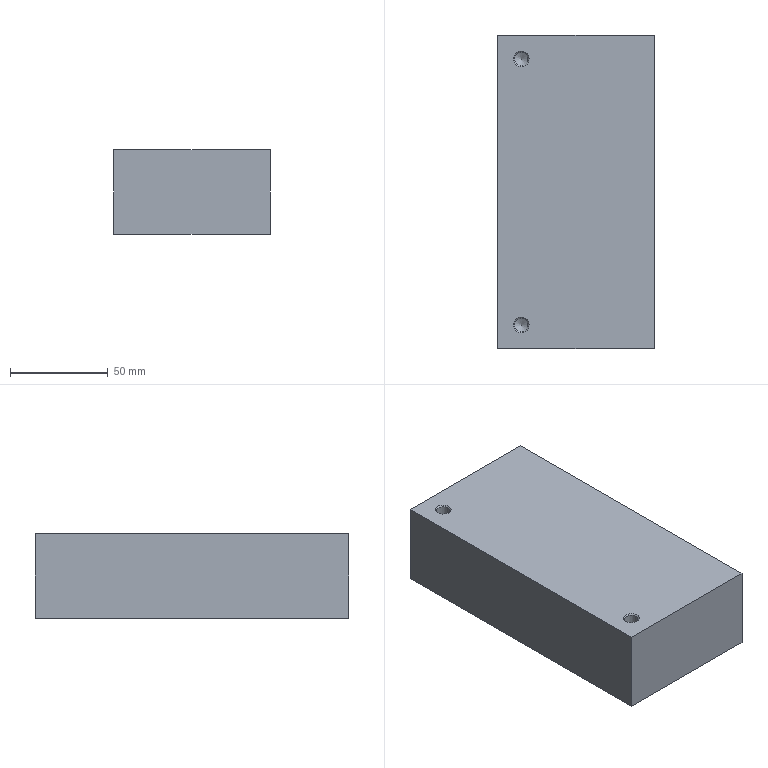Part | STEP file | 1 solid | 12 faces | box 80 x 160 x 43.2 mm | volume 550360 mm3 | plane 6 | cone 4 | cylinder 2 | commonest cylinder face diameters 6.8 x2
STEP:
#1=CARTESIAN_POINT('',(0.,0.,0.));
#2=DIRECTION('',(0.,0.,1.));
#3=DIRECTION('',(1.,0.,0.));
#4=AXIS2_PLACEMENT_3D('',#1,#2,#3);
#5=CARTESIAN_POINT('',(1856.247,362.48,-19.581));
#6=VERTEX_POINT('',#5);
#7=CARTESIAN_POINT('',(1936.247,362.48,-19.581));
#8=VERTEX_POINT('',#7);
#9=CARTESIAN_POINT('',(1956.247,362.48,-19.581));
#10=DIRECTION('',(1.,0.,0.));
#11=VECTOR('',#10,1.);
#12=LINE('',#9,#11);
#13=CARTESIAN_POINT('',(1806.549,562.98,-19.581));
#14=DIRECTION('',(0.,0.,-1.));
#15=DIRECTION('',(-1.,0.,0.));
#16=AXIS2_PLACEMENT_3D('',#13,#14,#15);
#17=PLANE('',#16);
#18=CARTESIAN_POINT('',(-149.698,-200.5));
#19=DIRECTION('',(-1.,0.));
#20=VECTOR('',#19,1.);
#21=LINE('',#18,#20);
#22=(GEOMETRIC_REPRESENTATION_CONTEXT(2)PARAMETRIC_REPRESENTATION_CONTEXT()REPRESENTATION_CONTEXT('',''));
#23=DEFINITIONAL_REPRESENTATION('',(#21),#22);
#24=PCURVE('',#17,#23);
#25=CARTESIAN_POINT('',(1956.247,362.48,23.619));
#26=DIRECTION('',(0.,-1.,0.));
#27=DIRECTION('',(0.,0.,1.));
#28=AXIS2_PLACEMENT_3D('',#25,#26,#27);
#29=PLANE('',#28);
#30=CARTESIAN_POINT('',(-43.2,0.));
#31=DIRECTION('',(0.,-1.));
#32=VECTOR('',#31,1.);
#33=LINE('',#30,#32);
#34=(GEOMETRIC_REPRESENTATION_CONTEXT(2)PARAMETRIC_REPRESENTATION_CONTEXT()REPRESENTATION_CONTEXT('',''));
#35=DEFINITIONAL_REPRESENTATION('',(#33),#34);
#36=PCURVE('',#29,#35);
#37=SURFACE_CURVE('',#12,(#24,#36),.PCURVE_S1.);
#38=EDGE_CURVE('',#6,#8,#37,.T.);
#39=ORIENTED_EDGE('',*,*,#38,.F.);
#40=CARTESIAN_POINT('',(1856.247,522.48,-19.581));
#41=VERTEX_POINT('',#40);
#42=CARTESIAN_POINT('',(1856.247,392.48,-19.581));
#43=DIRECTION('',(0.,-1.,0.));
#44=VECTOR('',#43,1.);
#45=LINE('',#42,#44);
#46=CARTESIAN_POINT('',(-49.698,-170.5));
#47=DIRECTION('',(0.,-1.));
#48=VECTOR('',#47,1.);
#49=LINE('',#46,#48);
#50=(GEOMETRIC_REPRESENTATION_CONTEXT(2)PARAMETRIC_REPRESENTATION_CONTEXT()REPRESENTATION_CONTEXT('',''));
#51=DEFINITIONAL_REPRESENTATION('',(#49),#50);
#52=PCURVE('',#17,#51);
#53=CARTESIAN_POINT('',(1856.247,392.48,23.619));
#54=DIRECTION('',(-1.,0.,0.));
#55=DIRECTION('',(0.,0.,1.));
#56=AXIS2_PLACEMENT_3D('',#53,#54,#55);
#57=PLANE('',#56);
#58=CARTESIAN_POINT('',(-43.2,0.));
#59=DIRECTION('',(0.,-1.));
#60=VECTOR('',#59,1.);
#61=LINE('',#58,#60);
#62=(GEOMETRIC_REPRESENTATION_CONTEXT(2)PARAMETRIC_REPRESENTATION_CONTEXT()REPRESENTATION_CONTEXT('',''));
#63=DEFINITIONAL_REPRESENTATION('',(#61),#62);
#64=PCURVE('',#57,#63);
#65=SURFACE_CURVE('',#45,(#52,#64),.PCURVE_S1.);
#66=EDGE_CURVE('',#41,#6,#65,.T.);
#67=ORIENTED_EDGE('',*,*,#66,.F.);
#68=CARTESIAN_POINT('',(1936.247,522.48,-19.581));
#69=VERTEX_POINT('',#68);
#70=CARTESIAN_POINT('',(1856.247,522.48,-19.581));
#71=DIRECTION('',(-1.,0.,0.));
#72=VECTOR('',#71,1.);
#73=LINE('',#70,#72);
#74=CARTESIAN_POINT('',(-49.698,-40.5));
#75=DIRECTION('',(1.,0.));
#76=VECTOR('',#75,1.);
#77=LINE('',#74,#76);
#78=(GEOMETRIC_REPRESENTATION_CONTEXT(2)PARAMETRIC_REPRESENTATION_CONTEXT()REPRESENTATION_CONTEXT('',''));
#79=DEFINITIONAL_REPRESENTATION('',(#77),#78);
#80=PCURVE('',#17,#79);
#81=CARTESIAN_POINT('',(1856.247,522.48,23.619));
#82=DIRECTION('',(0.,1.,0.));
#83=DIRECTION('',(0.,0.,-1.));
#84=AXIS2_PLACEMENT_3D('',#81,#82,#83);
#85=PLANE('',#84);
#86=CARTESIAN_POINT('',(43.2,0.));
#87=DIRECTION('',(0.,1.));
#88=VECTOR('',#87,1.);
#89=LINE('',#86,#88);
#90=(GEOMETRIC_REPRESENTATION_CONTEXT(2)PARAMETRIC_REPRESENTATION_CONTEXT()REPRESENTATION_CONTEXT('',''));
#91=DEFINITIONAL_REPRESENTATION('',(#89),#90);
#92=PCURVE('',#85,#91);
#93=SURFACE_CURVE('',#73,(#80,#92),.PCURVE_S1.);
#94=EDGE_CURVE('',#69,#41,#93,.T.);
#95=ORIENTED_EDGE('',*,*,#94,.F.);
#96=CARTESIAN_POINT('',(1936.247,492.48,-19.581));
#97=DIRECTION('',(0.,1.,0.));
#98=VECTOR('',#97,1.);
#99=LINE('',#96,#98);
#100=CARTESIAN_POINT('',(-129.698,-70.5));
#101=DIRECTION('',(0.,1.));
#102=VECTOR('',#101,1.);
#103=LINE('',#100,#102);
#104=(GEOMETRIC_REPRESENTATION_CONTEXT(2)PARAMETRIC_REPRESENTATION_CONTEXT()REPRESENTATION_CONTEXT('',''));
#105=DEFINITIONAL_REPRESENTATION('',(#103),#104);
#106=PCURVE('',#17,#105);
#107=CARTESIAN_POINT('',(1936.247,492.48,23.619));
#108=DIRECTION('',(1.,0.,0.));
#109=DIRECTION('',(0.,0.,-1.));
#110=AXIS2_PLACEMENT_3D('',#107,#108,#109);
#111=PLANE('',#110);
#112=CARTESIAN_POINT('',(43.2,0.));
#113=DIRECTION('',(0.,1.));
#114=VECTOR('',#113,1.);
#115=LINE('',#112,#114);
#116=(GEOMETRIC_REPRESENTATION_CONTEXT(2)PARAMETRIC_REPRESENTATION_CONTEXT()REPRESENTATION_CONTEXT('',''));
#117=DEFINITIONAL_REPRESENTATION('',(#115),#116);
#118=PCURVE('',#111,#117);
#119=SURFACE_CURVE('',#99,(#106,#118),.PCURVE_S1.);
#120=EDGE_CURVE('',#8,#69,#119,.T.);
#121=ORIENTED_EDGE('',*,*,#120,.F.);
#122=EDGE_LOOP('',(#39,#67,#95,#121));
#123=FACE_BOUND('',#122,.T.);
#124=ADVANCED_FACE('',(#123),#17,.T.);
#125=CARTESIAN_POINT('',(1856.247,522.48,23.619));
#126=VERTEX_POINT('',#125);
#127=CARTESIAN_POINT('',(1856.247,522.48,23.619));
#128=DIRECTION('',(0.,0.,-1.));
#129=VECTOR('',#128,1.);
#130=LINE('',#127,#129);
#131=CARTESIAN_POINT('',(0.,130.));
#132=DIRECTION('',(-1.,0.));
#133=VECTOR('',#132,1.);
#134=LINE('',#131,#133);
#135=(GEOMETRIC_REPRESENTATION_CONTEXT(2)PARAMETRIC_REPRESENTATION_CONTEXT()REPRESENTATION_CONTEXT('',''));
#136=DEFINITIONAL_REPRESENTATION('',(#134),#135);
#137=PCURVE('',#57,#136);
#138=CARTESIAN_POINT('',(0.,0.));
#139=DIRECTION('',(1.,0.));
#140=VECTOR('',#139,1.);
#141=LINE('',#138,#140);
#142=(GEOMETRIC_REPRESENTATION_CONTEXT(2)PARAMETRIC_REPRESENTATION_CONTEXT()REPRESENTATION_CONTEXT('',''));
#143=DEFINITIONAL_REPRESENTATION('',(#141),#142);
#144=PCURVE('',#85,#143);
#145=SURFACE_CURVE('',#130,(#137,#144),.PCURVE_S1.);
#146=EDGE_CURVE('',#126,#41,#145,.T.);
#147=ORIENTED_EDGE('',*,*,#146,.T.);
#148=ORIENTED_EDGE('',*,*,#66,.T.);
#149=CARTESIAN_POINT('',(1856.247,362.48,23.619));
#150=VERTEX_POINT('',#149);
#151=CARTESIAN_POINT('',(1856.247,362.48,23.619));
#152=DIRECTION('',(0.,0.,-1.));
#153=VECTOR('',#152,1.);
#154=LINE('',#151,#153);
#155=CARTESIAN_POINT('',(0.,-30.));
#156=DIRECTION('',(-1.,0.));
#157=VECTOR('',#156,1.);
#158=LINE('',#155,#157);
#159=(GEOMETRIC_REPRESENTATION_CONTEXT(2)PARAMETRIC_REPRESENTATION_CONTEXT()REPRESENTATION_CONTEXT('',''));
#160=DEFINITIONAL_REPRESENTATION('',(#158),#159);
#161=PCURVE('',#57,#160);
#162=CARTESIAN_POINT('',(0.,100.));
#163=DIRECTION('',(-1.,0.));
#164=VECTOR('',#163,1.);
#165=LINE('',#162,#164);
#166=(GEOMETRIC_REPRESENTATION_CONTEXT(2)PARAMETRIC_REPRESENTATION_CONTEXT()REPRESENTATION_CONTEXT('',''));
#167=DEFINITIONAL_REPRESENTATION('',(#165),#166);
#168=PCURVE('',#29,#167);
#169=SURFACE_CURVE('',#154,(#161,#168),.PCURVE_S1.);
#170=EDGE_CURVE('',#150,#6,#169,.T.);
#171=ORIENTED_EDGE('',*,*,#170,.F.);
#172=CARTESIAN_POINT('',(1856.247,392.48,23.619));
#173=DIRECTION('',(0.,1.,0.));
#174=VECTOR('',#173,1.);
#175=LINE('',#172,#174);
#176=CARTESIAN_POINT('',(0.,0.));
#177=DIRECTION('',(0.,1.));
#178=VECTOR('',#177,1.);
#179=LINE('',#176,#178);
#180=(GEOMETRIC_REPRESENTATION_CONTEXT(2)PARAMETRIC_REPRESENTATION_CONTEXT()REPRESENTATION_CONTEXT('',''));
#181=DEFINITIONAL_REPRESENTATION('',(#179),#180);
#182=PCURVE('',#57,#181);
#183=CARTESIAN_POINT('',(18457.433,-3577.789,23.619));
#184=DIRECTION('',(0.,0.,-1.));
#185=DIRECTION('',(-1.,0.,0.));
#186=AXIS2_PLACEMENT_3D('',#183,#184,#185);
#187=PLANE('',#186);
#188=CARTESIAN_POINT('',(16601.186,3970.269));
#189=DIRECTION('',(0.,1.));
#190=VECTOR('',#189,1.);
#191=LINE('',#188,#190);
#192=(GEOMETRIC_REPRESENTATION_CONTEXT(2)PARAMETRIC_REPRESENTATION_CONTEXT()REPRESENTATION_CONTEXT('',''));
#193=DEFINITIONAL_REPRESENTATION('',(#191),#192);
#194=PCURVE('',#187,#193);
#195=SURFACE_CURVE('',#175,(#182,#194),.PCURVE_S1.);
#196=EDGE_CURVE('',#150,#126,#195,.T.);
#197=ORIENTED_EDGE('',*,*,#196,.T.);
#198=EDGE_LOOP('',(#147,#148,#171,#197));
#199=FACE_BOUND('',#198,.T.);
#200=ADVANCED_FACE('',(#199),#57,.T.);
#201=CARTESIAN_POINT('',(1872.247,374.48,23.619));
#202=VERTEX_POINT('',#201);
#203=CARTESIAN_POINT('',(1868.247,374.48,23.619));
#204=DIRECTION('',(0.,0.,-1.));
#205=DIRECTION('',(1.,0.,0.));
#206=AXIS2_PLACEMENT_3D('',#203,#204,#205);
#207=CIRCLE('',#206,4.);
#208=CARTESIAN_POINT('',(16589.186,3952.269));
#209=DIRECTION('',(-1.,0.));
#210=AXIS2_PLACEMENT_2D('',#208,#209);
#211=CIRCLE('',#210,4.);
#212=(GEOMETRIC_REPRESENTATION_CONTEXT(2)PARAMETRIC_REPRESENTATION_CONTEXT()REPRESENTATION_CONTEXT('',''));
#213=DEFINITIONAL_REPRESENTATION('',(#211),#212);
#214=PCURVE('',#187,#213);
#215=CARTESIAN_POINT('',(1868.247,374.48,23.619));
#216=DIRECTION('',(0.,0.,1.));
#217=DIRECTION('',(1.,0.,0.));
#218=AXIS2_PLACEMENT_3D('',#215,#216,#217);
#219=CONICAL_SURFACE('',#218,4.,0.7854);
#220=CARTESIAN_POINT('',(6.283,0.));
#221=DIRECTION('',(-1.,0.));
#222=VECTOR('',#221,1.);
#223=LINE('',#220,#222);
#224=(GEOMETRIC_REPRESENTATION_CONTEXT(2)PARAMETRIC_REPRESENTATION_CONTEXT()REPRESENTATION_CONTEXT('',''));
#225=DEFINITIONAL_REPRESENTATION('',(#223),#224);
#226=PCURVE('',#219,#225);
#227=SURFACE_CURVE('',#207,(#214,#226),.PCURVE_S1.);
#228=EDGE_CURVE('',#202,#202,#227,.T.);
#229=ORIENTED_EDGE('',*,*,#228,.T.);
#230=EDGE_LOOP('',(#229));
#231=FACE_BOUND('',#230,.T.);
#232=CARTESIAN_POINT('',(1872.247,510.48,23.619));
#233=VERTEX_POINT('',#232);
#234=CARTESIAN_POINT('',(1868.247,510.48,23.619));
#235=DIRECTION('',(0.,0.,-1.));
#236=DIRECTION('',(1.,0.,0.));
#237=AXIS2_PLACEMENT_3D('',#234,#235,#236);
#238=CIRCLE('',#237,4.);
#239=CARTESIAN_POINT('',(16589.186,4088.269));
#240=DIRECTION('',(-1.,0.));
#241=AXIS2_PLACEMENT_2D('',#239,#240);
#242=CIRCLE('',#241,4.);
#243=(GEOMETRIC_REPRESENTATION_CONTEXT(2)PARAMETRIC_REPRESENTATION_CONTEXT()REPRESENTATION_CONTEXT('',''));
#244=DEFINITIONAL_REPRESENTATION('',(#242),#243);
#245=PCURVE('',#187,#244);
#246=CARTESIAN_POINT('',(1868.247,510.48,23.619));
#247=DIRECTION('',(0.,0.,1.));
#248=DIRECTION('',(1.,0.,0.));
#249=AXIS2_PLACEMENT_3D('',#246,#247,#248);
#250=CONICAL_SURFACE('',#249,4.,0.7854);
#251=CARTESIAN_POINT('',(6.283,0.));
#252=DIRECTION('',(-1.,0.));
#253=VECTOR('',#252,1.);
#254=LINE('',#251,#253);
#255=(GEOMETRIC_REPRESENTATION_CONTEXT(2)PARAMETRIC_REPRESENTATION_CONTEXT()REPRESENTATION_CONTEXT('',''));
#256=DEFINITIONAL_REPRESENTATION('',(#254),#255);
#257=PCURVE('',#250,#256);
#258=SURFACE_CURVE('',#238,(#245,#257),.PCURVE_S1.);
#259=EDGE_CURVE('',#233,#233,#258,.T.);
#260=ORIENTED_EDGE('',*,*,#259,.T.);
#261=EDGE_LOOP('',(#260));
#262=FACE_BOUND('',#261,.T.);
#263=CARTESIAN_POINT('',(1936.247,362.48,23.619));
#264=VERTEX_POINT('',#263);
#265=CARTESIAN_POINT('',(18457.433,362.48,23.619));
#266=DIRECTION('',(-1.,0.,0.));
#267=VECTOR('',#266,1.);
#268=LINE('',#265,#267);
#269=CARTESIAN_POINT('',(0.,3940.269));
#270=DIRECTION('',(1.,0.));
#271=VECTOR('',#270,1.);
#272=LINE('',#269,#271);
#273=(GEOMETRIC_REPRESENTATION_CONTEXT(2)PARAMETRIC_REPRESENTATION_CONTEXT()REPRESENTATION_CONTEXT('',''));
#274=DEFINITIONAL_REPRESENTATION('',(#272),#273);
#275=PCURVE('',#187,#274);
#276=CARTESIAN_POINT('',(0.,-16501.186));
#277=DIRECTION('',(0.,1.));
#278=VECTOR('',#277,1.);
#279=LINE('',#276,#278);
#280=(GEOMETRIC_REPRESENTATION_CONTEXT(2)PARAMETRIC_REPRESENTATION_CONTEXT()REPRESENTATION_CONTEXT('',''));
#281=DEFINITIONAL_REPRESENTATION('',(#279),#280);
#282=PCURVE('',#29,#281);
#283=SURFACE_CURVE('',#268,(#275,#282),.PCURVE_S1.);
#284=EDGE_CURVE('',#264,#150,#283,.T.);
#285=ORIENTED_EDGE('',*,*,#284,.F.);
#286=CARTESIAN_POINT('',(1936.247,522.48,23.619));
#287=VERTEX_POINT('',#286);
#288=CARTESIAN_POINT('',(1936.247,-3577.789,23.619));
#289=DIRECTION('',(0.,-1.,0.));
#290=VECTOR('',#289,1.);
#291=LINE('',#288,#290);
#292=CARTESIAN_POINT('',(16521.186,0.));
#293=DIRECTION('',(0.,-1.));
#294=VECTOR('',#293,1.);
#295=LINE('',#292,#294);
#296=(GEOMETRIC_REPRESENTATION_CONTEXT(2)PARAMETRIC_REPRESENTATION_CONTEXT()REPRESENTATION_CONTEXT('',''));
#297=DEFINITIONAL_REPRESENTATION('',(#295),#296);
#298=PCURVE('',#187,#297);
#299=CARTESIAN_POINT('',(0.,-4070.269));
#300=DIRECTION('',(0.,-1.));
#301=VECTOR('',#300,1.);
#302=LINE('',#299,#301);
#303=(GEOMETRIC_REPRESENTATION_CONTEXT(2)PARAMETRIC_REPRESENTATION_CONTEXT()REPRESENTATION_CONTEXT('',''));
#304=DEFINITIONAL_REPRESENTATION('',(#302),#303);
#305=PCURVE('',#111,#304);
#306=SURFACE_CURVE('',#291,(#298,#305),.PCURVE_S1.);
#307=EDGE_CURVE('',#287,#264,#306,.T.);
#308=ORIENTED_EDGE('',*,*,#307,.F.);
#309=CARTESIAN_POINT('',(18457.433,522.48,23.619));
#310=DIRECTION('',(1.,0.,0.));
#311=VECTOR('',#310,1.);
#312=LINE('',#309,#311);
#313=CARTESIAN_POINT('',(0.,4100.269));
#314=DIRECTION('',(-1.,0.));
#315=VECTOR('',#314,1.);
#316=LINE('',#313,#315);
#317=(GEOMETRIC_REPRESENTATION_CONTEXT(2)PARAMETRIC_REPRESENTATION_CONTEXT()REPRESENTATION_CONTEXT('',''));
#318=DEFINITIONAL_REPRESENTATION('',(#316),#317);
#319=PCURVE('',#187,#318);
#320=CARTESIAN_POINT('',(0.,-16601.186));
#321=DIRECTION('',(0.,-1.));
#322=VECTOR('',#321,1.);
#323=LINE('',#320,#322);
#324=(GEOMETRIC_REPRESENTATION_CONTEXT(2)PARAMETRIC_REPRESENTATION_CONTEXT()REPRESENTATION_CONTEXT('',''));
#325=DEFINITIONAL_REPRESENTATION('',(#323),#324);
#326=PCURVE('',#85,#325);
#327=SURFACE_CURVE('',#312,(#319,#326),.PCURVE_S1.);
#328=EDGE_CURVE('',#126,#287,#327,.T.);
#329=ORIENTED_EDGE('',*,*,#328,.F.);
#330=ORIENTED_EDGE('',*,*,#196,.F.);
#331=EDGE_LOOP('',(#285,#308,#329,#330));
#332=FACE_BOUND('',#331,.T.);
#333=ADVANCED_FACE('',(#231,#262,#332),#187,.F.);
#334=CARTESIAN_POINT('',(1936.247,522.48,23.619));
#335=DIRECTION('',(0.,0.,-1.));
#336=VECTOR('',#335,1.);
#337=LINE('',#334,#336);
#338=CARTESIAN_POINT('',(0.,-80.));
#339=DIRECTION('',(1.,0.));
#340=VECTOR('',#339,1.);
#341=LINE('',#338,#340);
#342=(GEOMETRIC_REPRESENTATION_CONTEXT(2)PARAMETRIC_REPRESENTATION_CONTEXT()REPRESENTATION_CONTEXT('',''));
#343=DEFINITIONAL_REPRESENTATION('',(#341),#342);
#344=PCURVE('',#85,#343);
#345=CARTESIAN_POINT('',(0.,30.));
#346=DIRECTION('',(1.,0.));
#347=VECTOR('',#346,1.);
#348=LINE('',#345,#347);
#349=(GEOMETRIC_REPRESENTATION_CONTEXT(2)PARAMETRIC_REPRESENTATION_CONTEXT()REPRESENTATION_CONTEXT('',''));
#350=DEFINITIONAL_REPRESENTATION('',(#348),#349);
#351=PCURVE('',#111,#350);
#352=SURFACE_CURVE('',#337,(#344,#351),.PCURVE_S1.);
#353=EDGE_CURVE('',#287,#69,#352,.T.);
#354=ORIENTED_EDGE('',*,*,#353,.T.);
#355=ORIENTED_EDGE('',*,*,#94,.T.);
#356=ORIENTED_EDGE('',*,*,#146,.F.);
#357=ORIENTED_EDGE('',*,*,#328,.T.);
#358=EDGE_LOOP('',(#354,#355,#356,#357));
#359=FACE_BOUND('',#358,.T.);
#360=ADVANCED_FACE('',(#359),#85,.T.);
#361=ORIENTED_EDGE('',*,*,#170,.T.);
#362=ORIENTED_EDGE('',*,*,#38,.T.);
#363=CARTESIAN_POINT('',(1936.247,362.48,23.619));
#364=DIRECTION('',(0.,0.,-1.));
#365=VECTOR('',#364,1.);
#366=LINE('',#363,#365);
#367=CARTESIAN_POINT('',(0.,20.));
#368=DIRECTION('',(-1.,0.));
#369=VECTOR('',#368,1.);
#370=LINE('',#367,#369);
#371=(GEOMETRIC_REPRESENTATION_CONTEXT(2)PARAMETRIC_REPRESENTATION_CONTEXT()REPRESENTATION_CONTEXT('',''));
#372=DEFINITIONAL_REPRESENTATION('',(#370),#371);
#373=PCURVE('',#29,#372);
#374=CARTESIAN_POINT('',(0.,-130.));
#375=DIRECTION('',(1.,0.));
#376=VECTOR('',#375,1.);
#377=LINE('',#374,#376);
#378=(GEOMETRIC_REPRESENTATION_CONTEXT(2)PARAMETRIC_REPRESENTATION_CONTEXT()REPRESENTATION_CONTEXT('',''));
#379=DEFINITIONAL_REPRESENTATION('',(#377),#378);
#380=PCURVE('',#111,#379);
#381=SURFACE_CURVE('',#366,(#373,#380),.PCURVE_S1.);
#382=EDGE_CURVE('',#264,#8,#381,.T.);
#383=ORIENTED_EDGE('',*,*,#382,.F.);
#384=ORIENTED_EDGE('',*,*,#284,.T.);
#385=EDGE_LOOP('',(#361,#362,#383,#384));
#386=FACE_BOUND('',#385,.T.);
#387=ADVANCED_FACE('',(#386),#29,.T.);
#388=ORIENTED_EDGE('',*,*,#382,.T.);
#389=ORIENTED_EDGE('',*,*,#120,.T.);
#390=ORIENTED_EDGE('',*,*,#353,.F.);
#391=ORIENTED_EDGE('',*,*,#307,.T.);
#392=EDGE_LOOP('',(#388,#389,#390,#391));
#393=FACE_BOUND('',#392,.T.);
#394=ADVANCED_FACE('',(#393),#111,.T.);
#395=CARTESIAN_POINT('',(1871.647,510.48,-11.381));
#396=VERTEX_POINT('',#395);
#397=CARTESIAN_POINT('',(1868.247,510.48,-11.381));
#398=DIRECTION('',(0.,0.,1.));
#399=DIRECTION('',(1.,0.,0.));
#400=AXIS2_PLACEMENT_3D('',#397,#398,#399);
#401=CIRCLE('',#400,3.4);
#402=CARTESIAN_POINT('',(1868.247,510.48,-11.381));
#403=DIRECTION('',(0.,0.,1.));
#404=DIRECTION('',(1.,0.,0.));
#405=AXIS2_PLACEMENT_3D('',#402,#403,#404);
#406=CONICAL_SURFACE('',#405,3.4,1.03);
#407=CARTESIAN_POINT('',(0.,0.));
#408=DIRECTION('',(1.,0.));
#409=VECTOR('',#408,1.);
#410=LINE('',#407,#409);
#411=(GEOMETRIC_REPRESENTATION_CONTEXT(2)PARAMETRIC_REPRESENTATION_CONTEXT()REPRESENTATION_CONTEXT('',''));
#412=DEFINITIONAL_REPRESENTATION('',(#410),#411);
#413=PCURVE('',#406,#412);
#414=CARTESIAN_POINT('',(1868.247,510.48,23.619));
#415=DIRECTION('',(0.,0.,-1.));
#416=DIRECTION('',(-1.,0.,0.));
#417=AXIS2_PLACEMENT_3D('',#414,#415,#416);
#418=CYLINDRICAL_SURFACE('',#417,3.4);
#419=CARTESIAN_POINT('',(9.425,35.));
#420=DIRECTION('',(-1.,0.));
#421=VECTOR('',#420,1.);
#422=LINE('',#419,#421);
#423=(GEOMETRIC_REPRESENTATION_CONTEXT(2)PARAMETRIC_REPRESENTATION_CONTEXT()REPRESENTATION_CONTEXT('',''));
#424=DEFINITIONAL_REPRESENTATION('',(#422),#423);
#425=PCURVE('',#418,#424);
#426=SURFACE_CURVE('',#401,(#413,#425),.PCURVE_S1.);
#427=EDGE_CURVE('',#396,#396,#426,.T.);
#428=ORIENTED_EDGE('',*,*,#427,.F.);
#429=CARTESIAN_POINT('',(1868.247,510.48,-13.424));
#430=VERTEX_POINT('',#429);
#431=CARTESIAN_POINT('',(1868.247,510.48,-13.424));
#432=CARTESIAN_POINT('',(1871.647,510.48,-11.381));
#433=B_SPLINE_CURVE_WITH_KNOTS('',1,(#431,#432),.UNSPECIFIED.,.F.,.F.,(2,2),(-3.967,0.),.PIECEWISE_BEZIER_KNOTS.);
#434=CARTESIAN_POINT('',(0.,0.));
#435=DIRECTION('',(0.,1.));
#436=VECTOR('',#435,1.);
#437=LINE('',#434,#436);
#438=(GEOMETRIC_REPRESENTATION_CONTEXT(2)PARAMETRIC_REPRESENTATION_CONTEXT()REPRESENTATION_CONTEXT('',''));
#439=DEFINITIONAL_REPRESENTATION('',(#437),#438);
#440=PCURVE('',#406,#439);
#441=CARTESIAN_POINT('',(6.283,0.));
#442=DIRECTION('',(0.,1.));
#443=VECTOR('',#442,1.);
#444=LINE('',#441,#443);
#445=(GEOMETRIC_REPRESENTATION_CONTEXT(2)PARAMETRIC_REPRESENTATION_CONTEXT()REPRESENTATION_CONTEXT('',''));
#446=DEFINITIONAL_REPRESENTATION('',(#444),#445);
#447=PCURVE('',#406,#446);
#448=SEAM_CURVE('',#433,(#440,#447),.PCURVE_S1.);
#449=EDGE_CURVE('',#430,#396,#448,.T.);
#450=ORIENTED_EDGE('',*,*,#449,.F.);
#451=ORIENTED_EDGE('',*,*,#449,.T.);
#452=EDGE_LOOP('',(#428,#450,#451));
#453=FACE_BOUND('',#452,.F.);
#454=ADVANCED_FACE('',(#453),#406,.F.);
#455=CARTESIAN_POINT('',(1871.647,510.48,23.019));
#456=VERTEX_POINT('',#455);
#457=CARTESIAN_POINT('',(1868.247,510.48,23.019));
#458=DIRECTION('',(0.,0.,1.));
#459=DIRECTION('',(1.,0.,0.));
#460=AXIS2_PLACEMENT_3D('',#457,#458,#459);
#461=CIRCLE('',#460,3.4);
#462=CARTESIAN_POINT('',(9.425,0.6));
#463=DIRECTION('',(-1.,0.));
#464=VECTOR('',#463,1.);
#465=LINE('',#462,#464);
#466=(GEOMETRIC_REPRESENTATION_CONTEXT(2)PARAMETRIC_REPRESENTATION_CONTEXT()REPRESENTATION_CONTEXT('',''));
#467=DEFINITIONAL_REPRESENTATION('',(#465),#466);
#468=PCURVE('',#418,#467);
#469=CARTESIAN_POINT('',(0.,-0.6));
#470=DIRECTION('',(1.,0.));
#471=VECTOR('',#470,1.);
#472=LINE('',#469,#471);
#473=(GEOMETRIC_REPRESENTATION_CONTEXT(2)PARAMETRIC_REPRESENTATION_CONTEXT()REPRESENTATION_CONTEXT('',''));
#474=DEFINITIONAL_REPRESENTATION('',(#472),#473);
#475=PCURVE('',#250,#474);
#476=SURFACE_CURVE('',#461,(#468,#475),.PCURVE_S1.);
#477=EDGE_CURVE('',#456,#456,#476,.T.);
#478=ORIENTED_EDGE('',*,*,#477,.F.);
#479=CARTESIAN_POINT('',(1871.647,510.48,23.019));
#480=CARTESIAN_POINT('',(1871.647,510.48,-11.381));
#481=B_SPLINE_CURVE_WITH_KNOTS('',1,(#479,#480),.UNSPECIFIED.,.F.,.F.,(2,2),(0.6,35.),.PIECEWISE_BEZIER_KNOTS.);
#482=CARTESIAN_POINT('',(9.425,0.));
#483=DIRECTION('',(0.,1.));
#484=VECTOR('',#483,1.);
#485=LINE('',#482,#484);
#486=(GEOMETRIC_REPRESENTATION_CONTEXT(2)PARAMETRIC_REPRESENTATION_CONTEXT()REPRESENTATION_CONTEXT('',''));
#487=DEFINITIONAL_REPRESENTATION('',(#485),#486);
#488=PCURVE('',#418,#487);
#489=CARTESIAN_POINT('',(3.142,0.));
#490=DIRECTION('',(0.,1.));
#491=VECTOR('',#490,1.);
#492=LINE('',#489,#491);
#493=(GEOMETRIC_REPRESENTATION_CONTEXT(2)PARAMETRIC_REPRESENTATION_CONTEXT()REPRESENTATION_CONTEXT('',''));
#494=DEFINITIONAL_REPRESENTATION('',(#492),#493);
#495=PCURVE('',#418,#494);
#496=SEAM_CURVE('',#481,(#488,#495),.PCURVE_S1.);
#497=EDGE_CURVE('',#456,#396,#496,.T.);
#498=ORIENTED_EDGE('',*,*,#497,.T.);
#499=ORIENTED_EDGE('',*,*,#427,.T.);
#500=ORIENTED_EDGE('',*,*,#497,.F.);
#501=EDGE_LOOP('',(#478,#498,#499,#500));
#502=FACE_BOUND('',#501,.F.);
#503=ADVANCED_FACE('',(#502),#418,.F.);
#504=ORIENTED_EDGE('',*,*,#477,.T.);
#505=CARTESIAN_POINT('',(1871.647,510.48,23.019));
#506=CARTESIAN_POINT('',(1872.247,510.48,23.619));
#507=B_SPLINE_CURVE_WITH_KNOTS('',1,(#505,#506),.UNSPECIFIED.,.F.,.F.,(2,2),(-0.8485,0.),.PIECEWISE_BEZIER_KNOTS.);
#508=CARTESIAN_POINT('',(6.283,0.));
#509=DIRECTION('',(0.,1.));
#510=VECTOR('',#509,1.);
#511=LINE('',#508,#510);
#512=(GEOMETRIC_REPRESENTATION_CONTEXT(2)PARAMETRIC_REPRESENTATION_CONTEXT()REPRESENTATION_CONTEXT('',''));
#513=DEFINITIONAL_REPRESENTATION('',(#511),#512);
#514=PCURVE('',#250,#513);
#515=CARTESIAN_POINT('',(0.,0.));
#516=DIRECTION('',(0.,1.));
#517=VECTOR('',#516,1.);
#518=LINE('',#515,#517);
#519=(GEOMETRIC_REPRESENTATION_CONTEXT(2)PARAMETRIC_REPRESENTATION_CONTEXT()REPRESENTATION_CONTEXT('',''));
#520=DEFINITIONAL_REPRESENTATION('',(#518),#519);
#521=PCURVE('',#250,#520);
#522=SEAM_CURVE('',#507,(#514,#521),.PCURVE_S1.);
#523=EDGE_CURVE('',#456,#233,#522,.T.);
#524=ORIENTED_EDGE('',*,*,#523,.T.);
#525=ORIENTED_EDGE('',*,*,#259,.T.);
#526=ORIENTED_EDGE('',*,*,#523,.F.);
#527=EDGE_LOOP('',(#504,#524,#525,#526));
#528=FACE_BOUND('',#527,.F.);
#529=ADVANCED_FACE('',(#528),#250,.F.);
#530=CARTESIAN_POINT('',(1871.647,374.48,-11.381));
#531=VERTEX_POINT('',#530);
#532=CARTESIAN_POINT('',(1868.247,374.48,-11.381));
#533=DIRECTION('',(0.,0.,1.));
#534=DIRECTION('',(1.,0.,0.));
#535=AXIS2_PLACEMENT_3D('',#532,#533,#534);
#536=CIRCLE('',#535,3.4);
#537=CARTESIAN_POINT('',(1868.247,374.48,-11.381));
#538=DIRECTION('',(0.,0.,1.));
#539=DIRECTION('',(1.,0.,0.));
#540=AXIS2_PLACEMENT_3D('',#537,#538,#539);
#541=CONICAL_SURFACE('',#540,3.4,1.03);
#542=CARTESIAN_POINT('',(0.,0.));
#543=DIRECTION('',(1.,0.));
#544=VECTOR('',#543,1.);
#545=LINE('',#542,#544);
#546=(GEOMETRIC_REPRESENTATION_CONTEXT(2)PARAMETRIC_REPRESENTATION_CONTEXT()REPRESENTATION_CONTEXT('',''));
#547=DEFINITIONAL_REPRESENTATION('',(#545),#546);
#548=PCURVE('',#541,#547);
#549=CARTESIAN_POINT('',(1868.247,374.48,23.619));
#550=DIRECTION('',(0.,0.,-1.));
#551=DIRECTION('',(-1.,0.,0.));
#552=AXIS2_PLACEMENT_3D('',#549,#550,#551);
#553=CYLINDRICAL_SURFACE('',#552,3.4);
#554=CARTESIAN_POINT('',(9.425,35.));
#555=DIRECTION('',(-1.,0.));
#556=VECTOR('',#555,1.);
#557=LINE('',#554,#556);
#558=(GEOMETRIC_REPRESENTATION_CONTEXT(2)PARAMETRIC_REPRESENTATION_CONTEXT()REPRESENTATION_CONTEXT('',''));
#559=DEFINITIONAL_REPRESENTATION('',(#557),#558);
#560=PCURVE('',#553,#559);
#561=SURFACE_CURVE('',#536,(#548,#560),.PCURVE_S1.);
#562=EDGE_CURVE('',#531,#531,#561,.T.);
#563=ORIENTED_EDGE('',*,*,#562,.F.);
#564=CARTESIAN_POINT('',(1868.247,374.48,-13.424));
#565=VERTEX_POINT('',#564);
#566=CARTESIAN_POINT('',(1868.247,374.48,-13.424));
#567=CARTESIAN_POINT('',(1871.647,374.48,-11.381));
#568=B_SPLINE_CURVE_WITH_KNOTS('',1,(#566,#567),.UNSPECIFIED.,.F.,.F.,(2,2),(-3.967,0.),.PIECEWISE_BEZIER_KNOTS.);
#569=CARTESIAN_POINT('',(0.,0.));
#570=DIRECTION('',(0.,1.));
#571=VECTOR('',#570,1.);
#572=LINE('',#569,#571);
#573=(GEOMETRIC_REPRESENTATION_CONTEXT(2)PARAMETRIC_REPRESENTATION_CONTEXT()REPRESENTATION_CONTEXT('',''));
#574=DEFINITIONAL_REPRESENTATION('',(#572),#573);
#575=PCURVE('',#541,#574);
#576=CARTESIAN_POINT('',(6.283,0.));
#577=DIRECTION('',(0.,1.));
#578=VECTOR('',#577,1.);
#579=LINE('',#576,#578);
#580=(GEOMETRIC_REPRESENTATION_CONTEXT(2)PARAMETRIC_REPRESENTATION_CONTEXT()REPRESENTATION_CONTEXT('',''));
#581=DEFINITIONAL_REPRESENTATION('',(#579),#580);
#582=PCURVE('',#541,#581);
#583=SEAM_CURVE('',#568,(#575,#582),.PCURVE_S1.);
#584=EDGE_CURVE('',#565,#531,#583,.T.);
#585=ORIENTED_EDGE('',*,*,#584,.F.);
#586=ORIENTED_EDGE('',*,*,#584,.T.);
#587=EDGE_LOOP('',(#563,#585,#586));
#588=FACE_BOUND('',#587,.F.);
#589=ADVANCED_FACE('',(#588),#541,.F.);
#590=CARTESIAN_POINT('',(1871.647,374.48,23.019));
#591=VERTEX_POINT('',#590);
#592=CARTESIAN_POINT('',(1868.247,374.48,23.019));
#593=DIRECTION('',(0.,0.,1.));
#594=DIRECTION('',(1.,0.,0.));
#595=AXIS2_PLACEMENT_3D('',#592,#593,#594);
#596=CIRCLE('',#595,3.4);
#597=CARTESIAN_POINT('',(9.425,0.6));
#598=DIRECTION('',(-1.,0.));
#599=VECTOR('',#598,1.);
#600=LINE('',#597,#599);
#601=(GEOMETRIC_REPRESENTATION_CONTEXT(2)PARAMETRIC_REPRESENTATION_CONTEXT()REPRESENTATION_CONTEXT('',''));
#602=DEFINITIONAL_REPRESENTATION('',(#600),#601);
#603=PCURVE('',#553,#602);
#604=CARTESIAN_POINT('',(0.,-0.6));
#605=DIRECTION('',(1.,0.));
#606=VECTOR('',#605,1.);
#607=LINE('',#604,#606);
#608=(GEOMETRIC_REPRESENTATION_CONTEXT(2)PARAMETRIC_REPRESENTATION_CONTEXT()REPRESENTATION_CONTEXT('',''));
#609=DEFINITIONAL_REPRESENTATION('',(#607),#608);
#610=PCURVE('',#219,#609);
#611=SURFACE_CURVE('',#596,(#603,#610),.PCURVE_S1.);
#612=EDGE_CURVE('',#591,#591,#611,.T.);
#613=ORIENTED_EDGE('',*,*,#612,.F.);
#614=CARTESIAN_POINT('',(1871.647,374.48,23.019));
#615=CARTESIAN_POINT('',(1871.647,374.48,-11.381));
#616=B_SPLINE_CURVE_WITH_KNOTS('',1,(#614,#615),.UNSPECIFIED.,.F.,.F.,(2,2),(0.6,35.),.PIECEWISE_BEZIER_KNOTS.);
#617=CARTESIAN_POINT('',(9.425,0.));
#618=DIRECTION('',(0.,1.));
#619=VECTOR('',#618,1.);
#620=LINE('',#617,#619);
#621=(GEOMETRIC_REPRESENTATION_CONTEXT(2)PARAMETRIC_REPRESENTATION_CONTEXT()REPRESENTATION_CONTEXT('',''));
#622=DEFINITIONAL_REPRESENTATION('',(#620),#621);
#623=PCURVE('',#553,#622);
#624=CARTESIAN_POINT('',(3.142,0.));
#625=DIRECTION('',(0.,1.));
#626=VECTOR('',#625,1.);
#627=LINE('',#624,#626);
#628=(GEOMETRIC_REPRESENTATION_CONTEXT(2)PARAMETRIC_REPRESENTATION_CONTEXT()REPRESENTATION_CONTEXT('',''));
#629=DEFINITIONAL_REPRESENTATION('',(#627),#628);
#630=PCURVE('',#553,#629);
#631=SEAM_CURVE('',#616,(#623,#630),.PCURVE_S1.);
#632=EDGE_CURVE('',#591,#531,#631,.T.);
#633=ORIENTED_EDGE('',*,*,#632,.T.);
#634=ORIENTED_EDGE('',*,*,#562,.T.);
#635=ORIENTED_EDGE('',*,*,#632,.F.);
#636=EDGE_LOOP('',(#613,#633,#634,#635));
#637=FACE_BOUND('',#636,.F.);
#638=ADVANCED_FACE('',(#637),#553,.F.);
#639=ORIENTED_EDGE('',*,*,#612,.T.);
#640=CARTESIAN_POINT('',(1871.647,374.48,23.019));
#641=CARTESIAN_POINT('',(1872.247,374.48,23.619));
#642=B_SPLINE_CURVE_WITH_KNOTS('',1,(#640,#641),.UNSPECIFIED.,.F.,.F.,(2,2),(-0.8485,0.),.PIECEWISE_BEZIER_KNOTS.);
#643=CARTESIAN_POINT('',(6.283,0.));
#644=DIRECTION('',(0.,1.));
#645=VECTOR('',#644,1.);
#646=LINE('',#643,#645);
#647=(GEOMETRIC_REPRESENTATION_CONTEXT(2)PARAMETRIC_REPRESENTATION_CONTEXT()REPRESENTATION_CONTEXT('',''));
#648=DEFINITIONAL_REPRESENTATION('',(#646),#647);
#649=PCURVE('',#219,#648);
#650=CARTESIAN_POINT('',(0.,0.));
#651=DIRECTION('',(0.,1.));
#652=VECTOR('',#651,1.);
#653=LINE('',#650,#652);
#654=(GEOMETRIC_REPRESENTATION_CONTEXT(2)PARAMETRIC_REPRESENTATION_CONTEXT()REPRESENTATION_CONTEXT('',''));
#655=DEFINITIONAL_REPRESENTATION('',(#653),#654);
#656=PCURVE('',#219,#655);
#657=SEAM_CURVE('',#642,(#649,#656),.PCURVE_S1.);
#658=EDGE_CURVE('',#591,#202,#657,.T.);
#659=ORIENTED_EDGE('',*,*,#658,.T.);
#660=ORIENTED_EDGE('',*,*,#228,.T.);
#661=ORIENTED_EDGE('',*,*,#658,.F.);
#662=EDGE_LOOP('',(#639,#659,#660,#661));
#663=FACE_BOUND('',#662,.F.);
#664=ADVANCED_FACE('',(#663),#219,.F.);
#665=CLOSED_SHELL('',(#124,#200,#333,#360,#387,#394,#454,#503,#529,#589,#638,#664));
#666=MANIFOLD_SOLID_BREP('',#665);
#667=(LENGTH_UNIT()NAMED_UNIT(*)SI_UNIT(.MILLI.,.METRE.));
#668=UNCERTAINTY_MEASURE_WITH_UNIT(LENGTH_MEASURE(0.000005),#667,'','');
#669=(NAMED_UNIT(*)PLANE_ANGLE_UNIT()SI_UNIT($,.RADIAN.));
#670=(NAMED_UNIT(*)SI_UNIT($,.STERADIAN.)SOLID_ANGLE_UNIT());
#671=(GEOMETRIC_REPRESENTATION_CONTEXT(3)GLOBAL_UNCERTAINTY_ASSIGNED_CONTEXT((#668))GLOBAL_UNIT_ASSIGNED_CONTEXT((#667,#669,#670))REPRESENTATION_CONTEXT('',''));
#672=ADVANCED_BREP_SHAPE_REPRESENTATION('',(#4,#666),#671);